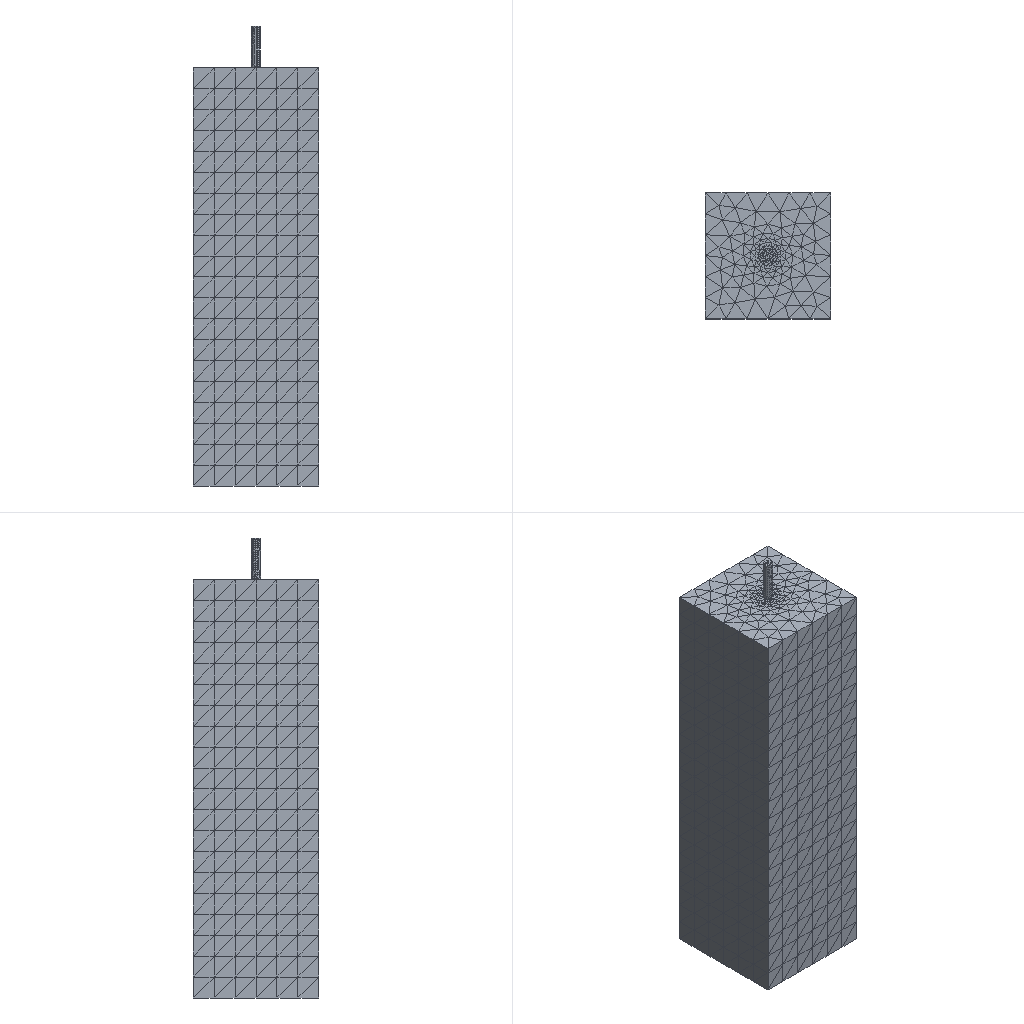Simulation study | abaqus
Set-up summary:
category,name,step,type,value,unit,region
solver,abaqus
solver,version,,,Abaqus/Standard 2020
units,not stated in the deck,,not stated
analysis,deck,,static,static
load_step,Step-1,Step-1,static
load_step,requested,,,1
mesh,nodes,,,120662
mesh,elements,,,80649
element_type,C3D10,,solid,80649
load,load commands in deck,,count,1
bc,support commands in deck,,count,3
material,MAO,,in results
material,SOIL,,in results
check,setup vs results,,match,"per instance, exact: element labels, types and connectivity; labels of the nodes the elements use; coordinates of those nodes at SINGLE_PRECISION in 2 of 2 instance(s)"
Abaqus input file, long lists of numbers shortened:
*Heading
** Job name: Job-2 Model name: Model-1-Copy
** Generated by: Abaqus/CAE 2020
*Preprint, echo=NO, model=NO, history=NO, contact=NO
**
** PARTS
**
*Part, name=merge-soil
*Node
      1,         150.,        -161.,         100.
      2,         150.,        -139.,         100.
** (86255 more lines like these left out)
*Element, type=C3D10
    1,  3425,  3426,  3427,  3428, 11554, 11553, 11552, 11556, 11555, 11557
    2,  3426,  3429,  3430,  3431, 11560, 11559, 11558, 11562, 11561, 11563
** (59732 more lines like these left out)
*Nset, nset=Set-4, generate
     1,  86257,      1
*Elset, elset=Set-4, generate
     1,  59734,      1
** Section: Section-1
*Solid Section, elset=Set-4, material=soil
,
*End Part
**
*Part, name=work
*Node
      1,   886.763,   1366.427,           5.
      2,   936.763,   1366.427,           5.
** (34403 more lines like these left out)
*Element, type=C3D10
   1, 3119, 3120, 3121, 3122, 5195, 5194, 5193, 5197, 5196, 5198
   2, 3119, 3123, 3122, 3124, 5200, 5199, 5197, 5202, 5201, 5203
** (20913 more lines like these left out)
*Nset, nset=Set-3, generate
     1,  34405,      1
*Elset, elset=Set-3, generate
     1,  20915,      1
** Section: Section-2
*Solid Section, elset=Set-3, material=mao
,
*End Part
**
**
** ASSEMBLY
**
*Assembly, name=Assembly
**
*Instance, name=work-1, part=work
        150.,  -1527.428,  -786.763
        150.,  -1527.428,  -786.763,         150., -1528.428,  -786.763, 90.
*End Instance
**
*Instance, name=merge-soil-1, part=merge-soil
*End Instance
**
*Node
      1,         150.,        -150.,        1100.
*Nset, nset=Set-7
 1,
*Nset, nset=Set-8, instance=merge-soil-1
    83,    84,    88,    89,   868,   869,   870,   871,   872,   946,   947,   948,   949,   950,   951,   952
   953,   954,   955,   956,   957,   958,   959,   960,  3080,  3081,  3082,  3083,  3084,  3085,  3086,  3087
** (9 more lines like these left out)
*Elset, elset=Set-8, instance=merge-soil-1
    27,   212,   546,   849,  1280,  5200,  5771,  5841,  5878,  5913,  5968,  6025, 13187, 13203, 22926, 22977
 23119, 23134, 23172, 23202, 23214, 25065, 25084, 25093, 25125, 25163, 25205, 25211, 25224, 25228, 25244, 25248
** (3 more lines like these left out)
*Nset, nset=Set-9, instance=merge-soil-1
    81,    82,    83,    84,    87,    88,    89,    90,   844,   845,   846,   847,   848,   849,   850,   851
   852,   853,   854,   855,   856,   857,   858,   859,   860,   861,   862,   863,   864,   865,   866,   867
** (65 more lines like these left out)
*Elset, elset=Set-9, instance=merge-soil-1
    30,   202,   218,   255,   258,   411,   426,   502,   686,   720,   752,   759,   847,   968,  1178,  1188
  1591,  1840,  2023,  2037,  2267,  2277,  2485,  2521,  2848,  2934,  2935,  2981,  3281,  3794,  4147,  4233
** (28 more lines like these left out)
*Nset, nset=Set-10, instance=merge-soil-1
    81,    82,    83,    84,    87,    88,    89,    90,   849,   850,   851,   852,   853,   854,   855,   856
   857,   858,   859,   860,   861,   862,   863,   864,   865,   866,   867,   873,   874,   875,   876,   877
** (65 more lines like these left out)
*Elset, elset=Set-10, instance=merge-soil-1
   533,   571,   768,  1469,  1624,  1671,  1711,  1899,  1906,  1948,  2270,  2504,  2787,  3057,  3059,  3220
  3593,  3799,  4011,  4339,  4666,  4721,  4969,  5109,  5164,  5190,  5261,  5308,  5313,  5331,  5460,  5479
** (28 more lines like these left out)
*Nset, nset=m_Set-6
 1,
*Elset, elset=_m_Surf-2_S3, internal, instance=work-1
    16,    31,    33,    36,    37,    43,    51,    77,   114,   122,   137,   184,   217,   220,   242,   263
   267,   273,   286,   287,   305,   326,   328,   333,   356,   375,   382,   386,   388,   397,   399,   411
** (253 more lines like these left out)
*Elset, elset=_m_Surf-2_S2, internal, instance=work-1
   874,  1188,  1271,  1350,  1376,  1553,  1578,  1580,  1596,  1628,  1629,  1635,  1714,  1795,  1800,  1887
  1899,  2095,  2106,  2137,  2278,  2593,  3147,  3220,  3276,  3295,  3324,  3365,  3377,  3390,  3409,  3421
** (51 more lines like these left out)
*Elset, elset=_m_Surf-2_S4, internal, instance=work-1
     3,    17,   488,   576,   677,   878,  1063,  1089,  1212,  1216,  1293,  1299,  1310,  1337,  1364,  1463
  1508,  1540,  1598,  1604,  1629,  1688,  1748,  1755,  1856,  1981,  2018,  2037,  2074,  2096,  2129,  2137
** (22 more lines like these left out)
*Elset, elset=_m_Surf-2_S1, internal, instance=work-1
    94,   427,   487,   557,   632,   677,   950,  1035,  1047,  1048,  1106,  1188,  1251,  1269,  1293,  1364
  1421,  1480,  1585,  1629,  1703,  1748,  1850,  1856,  2090,  2696,  2897,  2992,  3001,  3085,  3098,  3139
** (54 more lines like these left out)
*Surface, type=ELEMENT, name=m_Surf-2
_m_Surf-2_S3, S3
_m_Surf-2_S2, S2
_m_Surf-2_S4, S4
_m_Surf-2_S1, S1
*Elset, elset=_s_Surf-1_S3, internal, instance=work-1
  4332,  5944,  5949,  5980,  6411,  6437,  6447,  6458,  6462,  6464,  6465,  6476,  6477,  6483,  6490,  6492
  6494,  6655,  6656,  6657,  6658,  6661,  6665,  6673,  6674,  6675,  6690,  6697,  7362, 18644
*Elset, elset=_s_Surf-1_S4, internal, instance=work-1
 4674,
*Elset, elset=_s_Surf-1_S1, internal, instance=work-1
 7233,
*Surface, type=ELEMENT, name=s_Surf-1
_s_Surf-1_S3, S3
_s_Surf-1_S4, S4
_s_Surf-1_S1, S1
*Elset, elset=_s_Surf-4_S1, internal, instance=merge-soil-1
  1542,  3389,  5092,  5223,  5302,  5311,  5333,  5344,  5394,  5506,  5626,  5870,  5983,  6120,  6129,  6658
  6813,  6849,  6883,  6895,  6905,  6907,  6928,  6937,  6945,  7015,  7027,  7034,  7083,  7090,  7128,  7163
** (38 more lines like these left out)
*Elset, elset=_s_Surf-4_S3, internal, instance=merge-soil-1
   215,   284,   401,   677,   840,   945,   950,  1008,  1062,  1542,  1674,  1709,  1710,  1778,  2128,  2428
  2514,  2712,  2837,  2920,  2969,  3157,  3198,  3214,  3271,  3390,  3578,  3648,  3798,  4336,  4430,  4546
** (243 more lines like these left out)
*Elset, elset=_s_Surf-4_S4, internal, instance=merge-soil-1
  1523,  3656,  5293,  5453,  5511,  5569,  5628,  5650,  5673,  5677,  5773,  5778,  5983,  5998,  6067,  6094
  6125,  6141,  6190,  6353,  6430,  6437,  6448,  6975,  6978,  7053,  7090,  7132,  7297,  7452,  7475,  7497
** (22 more lines like these left out)
*Elset, elset=_s_Surf-4_S2, internal, instance=merge-soil-1
   133,   503,  1774,  2026,  2562,  5086,  5094,  5155,  5178,  5518,  5624,  5628,  5677,  5941,  6049,  6231
  6258,  6307,  6353,  6414,  6511,  6557,  6591,  6595,  6600,  6751,  6753,  6769,  6778,  6785,  6792,  6802
** (36 more lines like these left out)
*Surface, type=ELEMENT, name=s_Surf-4
_s_Surf-4_S1, S1
_s_Surf-4_S3, S3
_s_Surf-4_S4, S4
_s_Surf-4_S2, S2
** Constraint: Constraint-1
*Coupling, constraint name=Constraint-1, ref node=m_Set-6, surface=s_Surf-1
*Kinematic
*End Assembly
*Amplitude, name=Amp-1
             0.,              0.,              1.,              1.
**
** MATERIALS
**
*Material, name=mao
*Density
 7.8e-09,
*Elastic
140000., 0.32
*Plastic
348.,0.
*Material, name=soil
*Density
 2.7e-09,
*Elastic
5100., 0.25
*Mohr Coulomb
32., 0.1
*Mohr Coulomb Hardening
 4.6,0.
**
** INTERACTION PROPERTIES
**
*Surface Interaction, name=IntProp-1
1.,
*Friction, slip tolerance=0.005
 0.2,
*Surface Behavior, pressure-overclosure=HARD
**
** BOUNDARY CONDITIONS
**
** Name: BC-1 Type: 对称/反对称/完全固定
*Boundary
Set-8, ENCASTRE
** Name: BC-2 Type: 位移/转角
*Boundary
Set-10, 2, 2
** Name: BC-3 Type: 位移/转角
*Boundary
Set-9, 1, 1
**
** INTERACTIONS
**
** Interaction: Int-1
*Contact Pair, interaction=IntProp-1, type=SURFACE TO SURFACE
s_Surf-4, m_Surf-2
** ----------------------------------------------------------------
**
** STEP: Step-1
**
*Step, name=Step-1, nlgeom=YES, inc=1000
*Static, stabilize=0.0002, allsdtol=0.05, continue=NO
0.01, 1., 1e-05, 1.
**
** LOADS
**
** Name: Load-1   Type: Concentrated force
*Cload, amplitude=Amp-1
Set-7, 3, 100000.
**
** OUTPUT REQUESTS
**
*Restart, write, frequency=0
**
** FIELD OUTPUT: F-Output-1
**
*Output, field
*Node Output
CF, RF, RM, RT, TF, U, V
*Element Output, directions=YES
E, LE, MISES, MISESMAX, MISESONLY, PE, PEEQ, PEMAG, S, SF, SSAVG
*Contact Output
CDISP, CFORCE, CSTATUS, CSTRESS
**
** HISTORY OUTPUT: H-Output-1
**
*Output, history
*Node Output, nset=Set-7
U3, V3
*End Step
Results summary:
result,step,,partial,increments=5 time=0.01648/1.0
result,analysis,,,static
result,last_loadstep,,,1
result,primary field,,,U
result,reaction total,,FX,0.004112,model units
result,reaction total,,FY,-0.002773,model units
result,reaction total,,FZ,-1300.993,model units